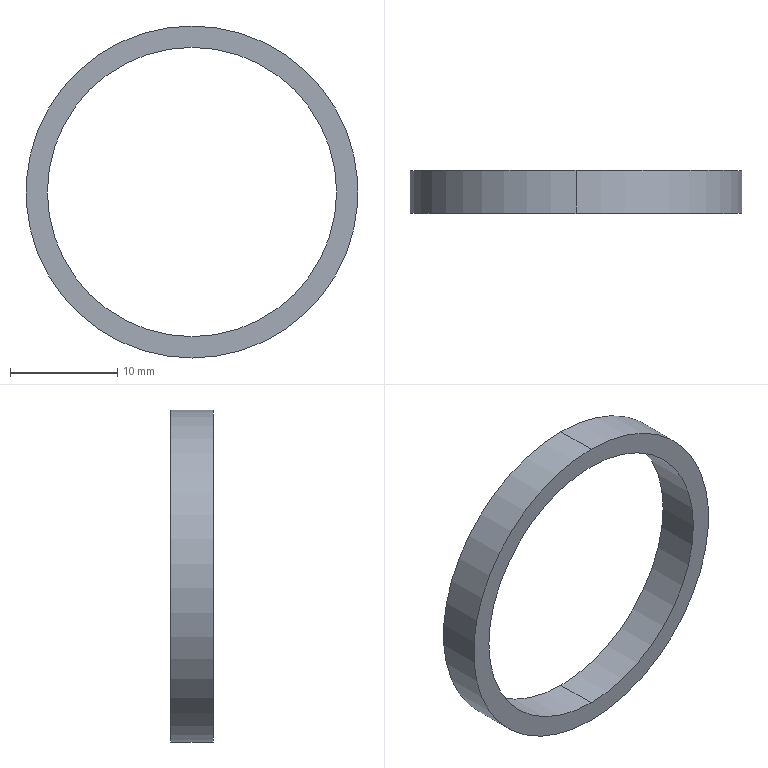Part | SolidWorks | features Revolution 1 | 1 solid | 6 faces | box 31 x 4 x 31 mm | volume 728.849 mm3 | cylinder 4 | plane 2 | commonest cylinder face diameters 27 x2 31 x2
STEP:
#1=CARTESIAN_POINT('',(0.,4.,-15.5));
#2=VERTEX_POINT('',#1);
#3=CARTESIAN_POINT('',(0.,4.,15.5));
#4=VERTEX_POINT('',#3);
#5=CARTESIAN_POINT('',(0.,4.,0.));
#6=DIRECTION('',(0.,-1.,0.));
#7=DIRECTION('',(0.,0.,-1.));
#8=AXIS2_PLACEMENT_3D('',#5,#6,#7);
#9=CIRCLE('',#8,15.5);
#10=EDGE_CURVE('',#2,#4,#9,.T.);
#11=ORIENTED_EDGE('',*,*,#10,.T.);
#12=CARTESIAN_POINT('',(0.,0.,15.5));
#13=VERTEX_POINT('',#12);
#14=CARTESIAN_POINT('',(0.,-1.541,15.5));
#15=DIRECTION('',(0.,-1.,0.));
#16=VECTOR('',#15,1000.);
#17=LINE('',#14,#16);
#18=EDGE_CURVE('',#4,#13,#17,.T.);
#19=ORIENTED_EDGE('',*,*,#18,.T.);
#20=CARTESIAN_POINT('',(0.,0.,-15.5));
#21=VERTEX_POINT('',#20);
#22=CARTESIAN_POINT('',(0.,0.,0.));
#23=DIRECTION('',(0.,-1.,0.));
#24=DIRECTION('',(0.,0.,-1.));
#25=AXIS2_PLACEMENT_3D('',#22,#23,#24);
#26=CIRCLE('',#25,15.5);
#27=EDGE_CURVE('',#21,#13,#26,.T.);
#28=ORIENTED_EDGE('',*,*,#27,.F.);
#29=CARTESIAN_POINT('',(0.,-1.541,-15.5));
#30=DIRECTION('',(0.,-1.,0.));
#31=VECTOR('',#30,1000.);
#32=LINE('',#29,#31);
#33=EDGE_CURVE('',#2,#21,#32,.T.);
#34=ORIENTED_EDGE('',*,*,#33,.F.);
#35=EDGE_LOOP('',(#11,#19,#28,#34));
#36=FACE_OUTER_BOUND('',#35,.T.);
#37=CARTESIAN_POINT('',(0.,-1.541,0.));
#38=DIRECTION('',(0.,-1.,0.));
#39=DIRECTION('',(0.,0.,-1.));
#40=AXIS2_PLACEMENT_3D('',#37,#38,#39);
#41=CYLINDRICAL_SURFACE('',#40,15.5);
#42=ADVANCED_FACE('',(#36),#41,.T.);
#43=CARTESIAN_POINT('',(0.,4.,13.5));
#44=VERTEX_POINT('',#43);
#45=CARTESIAN_POINT('',(0.,4.,-13.5));
#46=VERTEX_POINT('',#45);
#47=CARTESIAN_POINT('',(0.,4.,0.));
#48=DIRECTION('',(0.,-1.,0.));
#49=DIRECTION('',(0.,0.,-1.));
#50=AXIS2_PLACEMENT_3D('',#47,#48,#49);
#51=CIRCLE('',#50,13.5);
#52=EDGE_CURVE('',#44,#46,#51,.T.);
#53=ORIENTED_EDGE('',*,*,#52,.F.);
#54=CARTESIAN_POINT('',(0.,0.,13.5));
#55=VERTEX_POINT('',#54);
#56=CARTESIAN_POINT('',(0.,-1.541,13.5));
#57=DIRECTION('',(0.,-1.,0.));
#58=VECTOR('',#57,1000.);
#59=LINE('',#56,#58);
#60=EDGE_CURVE('',#44,#55,#59,.T.);
#61=ORIENTED_EDGE('',*,*,#60,.T.);
#62=CARTESIAN_POINT('',(0.,0.,-13.5));
#63=VERTEX_POINT('',#62);
#64=CARTESIAN_POINT('',(0.,0.,0.));
#65=DIRECTION('',(0.,-1.,0.));
#66=DIRECTION('',(0.,0.,-1.));
#67=AXIS2_PLACEMENT_3D('',#64,#65,#66);
#68=CIRCLE('',#67,13.5);
#69=EDGE_CURVE('',#55,#63,#68,.T.);
#70=ORIENTED_EDGE('',*,*,#69,.T.);
#71=CARTESIAN_POINT('',(0.,-1.541,-13.5));
#72=DIRECTION('',(0.,-1.,0.));
#73=VECTOR('',#72,1000.);
#74=LINE('',#71,#73);
#75=EDGE_CURVE('',#46,#63,#74,.T.);
#76=ORIENTED_EDGE('',*,*,#75,.F.);
#77=EDGE_LOOP('',(#53,#61,#70,#76));
#78=FACE_OUTER_BOUND('',#77,.T.);
#79=CARTESIAN_POINT('',(0.,-1.541,0.));
#80=DIRECTION('',(0.,-1.,0.));
#81=DIRECTION('',(0.,0.,-1.));
#82=AXIS2_PLACEMENT_3D('',#79,#80,#81);
#83=CYLINDRICAL_SURFACE('',#82,13.5);
#84=ADVANCED_FACE('',(#78),#83,.F.);
#85=ORIENTED_EDGE('',*,*,#27,.T.);
#86=CARTESIAN_POINT('',(0.,0.,0.));
#87=DIRECTION('',(0.,-1.,0.));
#88=DIRECTION('',(0.,0.,-1.));
#89=AXIS2_PLACEMENT_3D('',#86,#87,#88);
#90=CIRCLE('',#89,15.5);
#91=EDGE_CURVE('',#13,#21,#90,.T.);
#92=ORIENTED_EDGE('',*,*,#91,.T.);
#93=EDGE_LOOP('',(#85,#92));
#94=FACE_OUTER_BOUND('',#93,.T.);
#95=CARTESIAN_POINT('',(0.,0.,0.));
#96=DIRECTION('',(0.,-1.,0.));
#97=DIRECTION('',(0.,0.,-1.));
#98=AXIS2_PLACEMENT_3D('',#95,#96,#97);
#99=CIRCLE('',#98,13.5);
#100=EDGE_CURVE('',#63,#55,#99,.T.);
#101=ORIENTED_EDGE('',*,*,#100,.F.);
#102=ORIENTED_EDGE('',*,*,#69,.F.);
#103=EDGE_LOOP('',(#101,#102));
#104=FACE_BOUND('',#103,.T.);
#105=CARTESIAN_POINT('',(15.5,0.,0.));
#106=DIRECTION('',(0.,-1.,0.));
#107=DIRECTION('',(0.,0.,-1.));
#108=AXIS2_PLACEMENT_3D('',#105,#106,#107);
#109=PLANE('',#108);
#110=ADVANCED_FACE('',(#94,#104),#109,.T.);
#111=ORIENTED_EDGE('',*,*,#60,.F.);
#112=CARTESIAN_POINT('',(0.,4.,0.));
#113=DIRECTION('',(0.,-1.,0.));
#114=DIRECTION('',(0.,0.,-1.));
#115=AXIS2_PLACEMENT_3D('',#112,#113,#114);
#116=CIRCLE('',#115,13.5);
#117=EDGE_CURVE('',#46,#44,#116,.T.);
#118=ORIENTED_EDGE('',*,*,#117,.F.);
#119=ORIENTED_EDGE('',*,*,#75,.T.);
#120=ORIENTED_EDGE('',*,*,#100,.T.);
#121=EDGE_LOOP('',(#111,#118,#119,#120));
#122=FACE_OUTER_BOUND('',#121,.T.);
#123=CARTESIAN_POINT('',(0.,-1.541,0.));
#124=DIRECTION('',(0.,-1.,0.));
#125=DIRECTION('',(0.,0.,-1.));
#126=AXIS2_PLACEMENT_3D('',#123,#124,#125);
#127=CYLINDRICAL_SURFACE('',#126,13.5);
#128=ADVANCED_FACE('',(#122),#127,.F.);
#129=ORIENTED_EDGE('',*,*,#117,.T.);
#130=ORIENTED_EDGE('',*,*,#52,.T.);
#131=EDGE_LOOP('',(#129,#130));
#132=FACE_BOUND('',#131,.T.);
#133=ORIENTED_EDGE('',*,*,#10,.F.);
#134=CARTESIAN_POINT('',(0.,4.,0.));
#135=DIRECTION('',(0.,-1.,0.));
#136=DIRECTION('',(0.,0.,-1.));
#137=AXIS2_PLACEMENT_3D('',#134,#135,#136);
#138=CIRCLE('',#137,15.5);
#139=EDGE_CURVE('',#4,#2,#138,.T.);
#140=ORIENTED_EDGE('',*,*,#139,.F.);
#141=EDGE_LOOP('',(#133,#140));
#142=FACE_OUTER_BOUND('',#141,.T.);
#143=CARTESIAN_POINT('',(13.5,4.,0.));
#144=DIRECTION('',(0.,1.,0.));
#145=DIRECTION('',(0.,0.,1.));
#146=AXIS2_PLACEMENT_3D('',#143,#144,#145);
#147=PLANE('',#146);
#148=ADVANCED_FACE('',(#132,#142),#147,.T.);
#149=ORIENTED_EDGE('',*,*,#18,.F.);
#150=ORIENTED_EDGE('',*,*,#139,.T.);
#151=ORIENTED_EDGE('',*,*,#33,.T.);
#152=ORIENTED_EDGE('',*,*,#91,.F.);
#153=EDGE_LOOP('',(#149,#150,#151,#152));
#154=FACE_OUTER_BOUND('',#153,.T.);
#155=CARTESIAN_POINT('',(0.,-1.541,0.));
#156=DIRECTION('',(0.,-1.,0.));
#157=DIRECTION('',(0.,0.,-1.));
#158=AXIS2_PLACEMENT_3D('',#155,#156,#157);
#159=CYLINDRICAL_SURFACE('',#158,15.5);
#160=ADVANCED_FACE('',(#154),#159,.T.);
#161=CLOSED_SHELL('',(#42,#84,#110,#128,#148,#160));
#162=MANIFOLD_SOLID_BREP('',#161);
#163=CARTESIAN_POINT('',(0.,0.,0.));
#164=DIRECTION('',(0.,0.,1.));
#165=DIRECTION('',(1.,0.,0.));
#166=AXIS2_PLACEMENT_3D('',#163,#164,#165);
#167=(LENGTH_UNIT()NAMED_UNIT(*)SI_UNIT(.MILLI.,.METRE.));
#168=UNCERTAINTY_MEASURE_WITH_UNIT(LENGTH_MEASURE(0.00001),#167,'','');
#169=(NAMED_UNIT(*)PLANE_ANGLE_UNIT()SI_UNIT($,.RADIAN.));
#170=(NAMED_UNIT(*)SI_UNIT($,.STERADIAN.)SOLID_ANGLE_UNIT());
#171=(GEOMETRIC_REPRESENTATION_CONTEXT(3)GLOBAL_UNCERTAINTY_ASSIGNED_CONTEXT((#168))GLOBAL_UNIT_ASSIGNED_CONTEXT((#167,#169,#170))REPRESENTATION_CONTEXT('',''));
#172=ADVANCED_BREP_SHAPE_REPRESENTATION('',(#162,#166),#171);